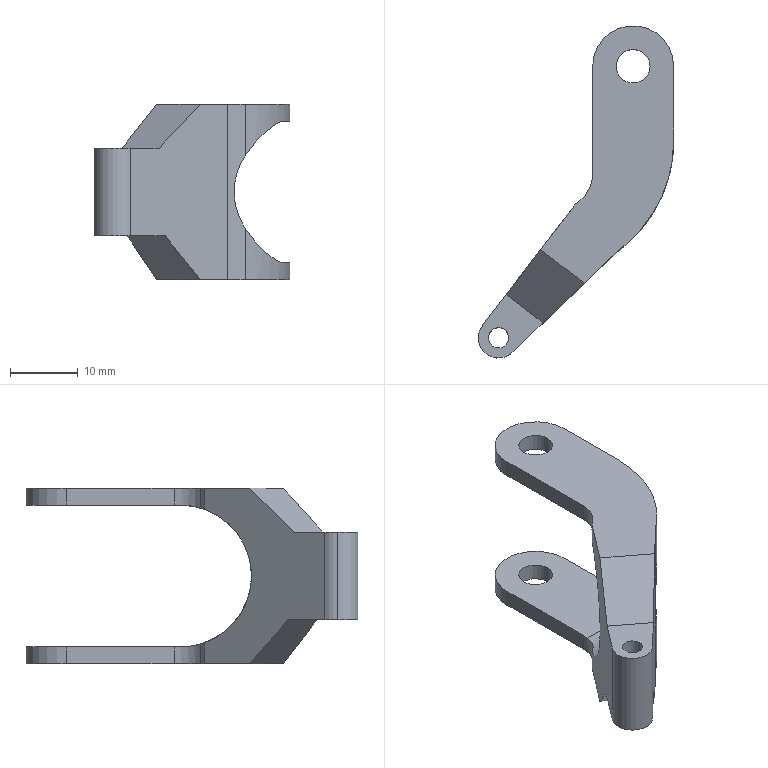Part | SolidWorks | features BaseBody 1 | 1 solid | 32 faces | box 28.933 x 49.206 x 26 mm | volume 4873 mm3 | plane 17 | cylinder 15 | commonest cylinder face diameters 5 x4 3 x2 6 x2 10 x2 12 x2 40 x2
STEP:
#1=CARTESIAN_POINT('',(6.042,20.411,23.5));
#2=VERTEX_POINT('',#1);
#3=CARTESIAN_POINT('',(11.042,20.411,23.5));
#4=VERTEX_POINT('',#3);
#5=CARTESIAN_POINT('',(8.542,20.411,23.5));
#6=DIRECTION('',(0.,0.,1.));
#7=DIRECTION('',(1.,0.,0.));
#8=AXIS2_PLACEMENT_3D('',#5,#6,#7);
#9=CIRCLE('',#8,2.5);
#10=EDGE_CURVE('',#2,#4,#9,.T.);
#11=ORIENTED_EDGE('',*,*,#10,.F.);
#12=CARTESIAN_POINT('',(6.042,20.411,26.));
#13=VERTEX_POINT('',#12);
#14=CARTESIAN_POINT('',(6.042,20.411,-34.));
#15=DIRECTION('',(0.,0.,1.));
#16=VECTOR('',#15,1000.);
#17=LINE('',#14,#16);
#18=EDGE_CURVE('',#2,#13,#17,.T.);
#19=ORIENTED_EDGE('',*,*,#18,.T.);
#20=CARTESIAN_POINT('',(11.042,20.411,26.));
#21=VERTEX_POINT('',#20);
#22=CARTESIAN_POINT('',(8.542,20.411,26.));
#23=DIRECTION('',(0.,0.,1.));
#24=DIRECTION('',(1.,0.,0.));
#25=AXIS2_PLACEMENT_3D('',#22,#23,#24);
#26=CIRCLE('',#25,2.5);
#27=EDGE_CURVE('',#13,#21,#26,.T.);
#28=ORIENTED_EDGE('',*,*,#27,.T.);
#29=CARTESIAN_POINT('',(11.042,20.411,-34.));
#30=DIRECTION('',(0.,0.,1.));
#31=VECTOR('',#30,1000.);
#32=LINE('',#29,#31);
#33=EDGE_CURVE('',#4,#21,#32,.T.);
#34=ORIENTED_EDGE('',*,*,#33,.F.);
#35=EDGE_LOOP('',(#11,#19,#28,#34));
#36=FACE_OUTER_BOUND('',#35,.T.);
#37=CARTESIAN_POINT('',(8.542,20.411,-34.));
#38=DIRECTION('',(0.,0.,1.));
#39=DIRECTION('',(1.,0.,0.));
#40=AXIS2_PLACEMENT_3D('',#37,#38,#39);
#41=CYLINDRICAL_SURFACE('',#40,2.5);
#42=ADVANCED_FACE('',(#36),#41,.F.);
#43=CARTESIAN_POINT('',(11.042,20.411,0.));
#44=VERTEX_POINT('',#43);
#45=CARTESIAN_POINT('',(6.042,20.411,0.));
#46=VERTEX_POINT('',#45);
#47=CARTESIAN_POINT('',(8.542,20.411,0.));
#48=DIRECTION('',(0.,0.,-1.));
#49=DIRECTION('',(-1.,0.,0.));
#50=AXIS2_PLACEMENT_3D('',#47,#48,#49);
#51=CIRCLE('',#50,2.5);
#52=EDGE_CURVE('',#44,#46,#51,.T.);
#53=ORIENTED_EDGE('',*,*,#52,.T.);
#54=CARTESIAN_POINT('',(6.042,20.411,2.5));
#55=VERTEX_POINT('',#54);
#56=CARTESIAN_POINT('',(6.042,20.411,-34.));
#57=DIRECTION('',(0.,0.,1.));
#58=VECTOR('',#57,1000.);
#59=LINE('',#56,#58);
#60=EDGE_CURVE('',#46,#55,#59,.T.);
#61=ORIENTED_EDGE('',*,*,#60,.T.);
#62=CARTESIAN_POINT('',(11.042,20.411,2.5));
#63=VERTEX_POINT('',#62);
#64=CARTESIAN_POINT('',(8.542,20.411,2.5));
#65=DIRECTION('',(0.,0.,-1.));
#66=DIRECTION('',(0.,1.,0.));
#67=AXIS2_PLACEMENT_3D('',#64,#65,#66);
#68=CIRCLE('',#67,2.5);
#69=EDGE_CURVE('',#63,#55,#68,.T.);
#70=ORIENTED_EDGE('',*,*,#69,.F.);
#71=CARTESIAN_POINT('',(11.042,20.411,-34.));
#72=DIRECTION('',(0.,0.,1.));
#73=VECTOR('',#72,1000.);
#74=LINE('',#71,#73);
#75=EDGE_CURVE('',#44,#63,#74,.T.);
#76=ORIENTED_EDGE('',*,*,#75,.F.);
#77=EDGE_LOOP('',(#53,#61,#70,#76));
#78=FACE_OUTER_BOUND('',#77,.T.);
#79=CARTESIAN_POINT('',(8.542,20.411,-34.));
#80=DIRECTION('',(0.,0.,1.));
#81=DIRECTION('',(1.,0.,0.));
#82=AXIS2_PLACEMENT_3D('',#79,#80,#81);
#83=CYLINDRICAL_SURFACE('',#82,2.5);
#84=ADVANCED_FACE('',(#78),#83,.F.);
#85=CARTESIAN_POINT('',(-12.891,-19.795,6.5));
#86=VERTEX_POINT('',#85);
#87=CARTESIAN_POINT('',(-9.891,-19.795,6.5));
#88=VERTEX_POINT('',#87);
#89=CARTESIAN_POINT('',(-11.391,-19.795,6.5));
#90=DIRECTION('',(0.,0.,1.));
#91=DIRECTION('',(1.,0.,0.));
#92=AXIS2_PLACEMENT_3D('',#89,#90,#91);
#93=CIRCLE('',#92,1.5);
#94=EDGE_CURVE('',#86,#88,#93,.T.);
#95=ORIENTED_EDGE('',*,*,#94,.F.);
#96=CARTESIAN_POINT('',(-12.891,-19.795,19.5));
#97=VERTEX_POINT('',#96);
#98=CARTESIAN_POINT('',(-12.891,-19.795,-34.));
#99=DIRECTION('',(0.,0.,1.));
#100=VECTOR('',#99,1000.);
#101=LINE('',#98,#100);
#102=EDGE_CURVE('',#86,#97,#101,.T.);
#103=ORIENTED_EDGE('',*,*,#102,.T.);
#104=CARTESIAN_POINT('',(-9.891,-19.795,19.5));
#105=VERTEX_POINT('',#104);
#106=CARTESIAN_POINT('',(-11.391,-19.795,19.5));
#107=DIRECTION('',(0.,0.,-1.));
#108=DIRECTION('',(-1.,0.,0.));
#109=AXIS2_PLACEMENT_3D('',#106,#107,#108);
#110=CIRCLE('',#109,1.5);
#111=EDGE_CURVE('',#105,#97,#110,.T.);
#112=ORIENTED_EDGE('',*,*,#111,.F.);
#113=CARTESIAN_POINT('',(-9.891,-19.795,-34.));
#114=DIRECTION('',(0.,0.,1.));
#115=VECTOR('',#114,1000.);
#116=LINE('',#113,#115);
#117=EDGE_CURVE('',#88,#105,#116,.T.);
#118=ORIENTED_EDGE('',*,*,#117,.F.);
#119=EDGE_LOOP('',(#95,#103,#112,#118));
#120=FACE_OUTER_BOUND('',#119,.T.);
#121=CARTESIAN_POINT('',(-11.391,-19.795,-34.));
#122=DIRECTION('',(0.,0.,1.));
#123=DIRECTION('',(1.,0.,0.));
#124=AXIS2_PLACEMENT_3D('',#121,#122,#123);
#125=CYLINDRICAL_SURFACE('',#124,1.5);
#126=ADVANCED_FACE('',(#120),#125,.F.);
#127=CARTESIAN_POINT('',(-9.059,-21.682,19.5));
#128=VERTEX_POINT('',#127);
#129=CARTESIAN_POINT('',(-14.391,-19.795,19.5));
#130=VERTEX_POINT('',#129);
#131=CARTESIAN_POINT('',(-11.391,-19.795,19.5));
#132=DIRECTION('',(0.,0.,-1.));
#133=DIRECTION('',(-1.,0.,0.));
#134=AXIS2_PLACEMENT_3D('',#131,#132,#133);
#135=CIRCLE('',#134,3.);
#136=EDGE_CURVE('',#128,#130,#135,.T.);
#137=ORIENTED_EDGE('',*,*,#136,.T.);
#138=CARTESIAN_POINT('',(-14.391,-19.795,6.5));
#139=VERTEX_POINT('',#138);
#140=CARTESIAN_POINT('',(-14.391,-19.795,26.));
#141=DIRECTION('',(0.,0.,-1.));
#142=VECTOR('',#141,1000.);
#143=LINE('',#140,#142);
#144=EDGE_CURVE('',#130,#139,#143,.T.);
#145=ORIENTED_EDGE('',*,*,#144,.T.);
#146=CARTESIAN_POINT('',(-9.059,-21.682,6.5));
#147=VERTEX_POINT('',#146);
#148=CARTESIAN_POINT('',(-11.391,-19.795,6.5));
#149=DIRECTION('',(0.,0.,1.));
#150=DIRECTION('',(1.,0.,0.));
#151=AXIS2_PLACEMENT_3D('',#148,#149,#150);
#152=CIRCLE('',#151,3.);
#153=EDGE_CURVE('',#139,#147,#152,.T.);
#154=ORIENTED_EDGE('',*,*,#153,.T.);
#155=CARTESIAN_POINT('',(-9.059,-21.682,26.));
#156=DIRECTION('',(0.,0.,-1.));
#157=VECTOR('',#156,1000.);
#158=LINE('',#155,#157);
#159=EDGE_CURVE('',#128,#147,#158,.T.);
#160=ORIENTED_EDGE('',*,*,#159,.F.);
#161=EDGE_LOOP('',(#137,#145,#154,#160));
#162=FACE_OUTER_BOUND('',#161,.T.);
#163=CARTESIAN_POINT('',(-11.391,-19.795,26.));
#164=DIRECTION('',(0.,0.,-1.));
#165=DIRECTION('',(-1.,0.,0.));
#166=AXIS2_PLACEMENT_3D('',#163,#164,#165);
#167=CYLINDRICAL_SURFACE('',#166,3.);
#168=ADVANCED_FACE('',(#162),#167,.T.);
#169=CARTESIAN_POINT('',(14.542,9.306,26.));
#170=VERTEX_POINT('',#169);
#171=CARTESIAN_POINT('',(14.542,20.411,26.));
#172=VERTEX_POINT('',#171);
#173=CARTESIAN_POINT('',(14.542,20.411,26.));
#174=DIRECTION('',(0.,1.,0.));
#175=VECTOR('',#174,1000.);
#176=LINE('',#173,#175);
#177=EDGE_CURVE('',#170,#172,#176,.T.);
#178=ORIENTED_EDGE('',*,*,#177,.F.);
#179=CARTESIAN_POINT('',(14.542,9.306,23.5));
#180=VERTEX_POINT('',#179);
#181=CARTESIAN_POINT('',(14.542,9.306,26.));
#182=DIRECTION('',(0.,0.,-1.));
#183=VECTOR('',#182,1000.);
#184=LINE('',#181,#183);
#185=EDGE_CURVE('',#170,#180,#184,.T.);
#186=ORIENTED_EDGE('',*,*,#185,.T.);
#187=CARTESIAN_POINT('',(14.542,20.411,23.5));
#188=VERTEX_POINT('',#187);
#189=CARTESIAN_POINT('',(14.542,20.411,23.5));
#190=DIRECTION('',(0.,1.,0.));
#191=VECTOR('',#190,1000.);
#192=LINE('',#189,#191);
#193=EDGE_CURVE('',#180,#188,#192,.T.);
#194=ORIENTED_EDGE('',*,*,#193,.T.);
#195=CARTESIAN_POINT('',(14.542,20.411,26.));
#196=DIRECTION('',(0.,0.,-1.));
#197=VECTOR('',#196,1000.);
#198=LINE('',#195,#197);
#199=EDGE_CURVE('',#172,#188,#198,.T.);
#200=ORIENTED_EDGE('',*,*,#199,.F.);
#201=EDGE_LOOP('',(#178,#186,#194,#200));
#202=FACE_OUTER_BOUND('',#201,.T.);
#203=CARTESIAN_POINT('',(14.542,20.411,26.));
#204=DIRECTION('',(-1.,0.,0.));
#205=DIRECTION('',(0.,-1.,0.));
#206=AXIS2_PLACEMENT_3D('',#203,#204,#205);
#207=PLANE('',#206);
#208=ADVANCED_FACE('',(#202),#207,.F.);
#209=ORIENTED_EDGE('',*,*,#199,.T.);
#210=CARTESIAN_POINT('',(2.542,20.411,23.5));
#211=VERTEX_POINT('',#210);
#212=CARTESIAN_POINT('',(8.542,20.411,23.5));
#213=DIRECTION('',(0.,0.,1.));
#214=DIRECTION('',(1.,0.,0.));
#215=AXIS2_PLACEMENT_3D('',#212,#213,#214);
#216=CIRCLE('',#215,6.);
#217=EDGE_CURVE('',#188,#211,#216,.T.);
#218=ORIENTED_EDGE('',*,*,#217,.T.);
#219=CARTESIAN_POINT('',(2.542,20.411,26.));
#220=VERTEX_POINT('',#219);
#221=CARTESIAN_POINT('',(2.542,20.411,26.));
#222=DIRECTION('',(0.,0.,-1.));
#223=VECTOR('',#222,1000.);
#224=LINE('',#221,#223);
#225=EDGE_CURVE('',#220,#211,#224,.T.);
#226=ORIENTED_EDGE('',*,*,#225,.F.);
#227=CARTESIAN_POINT('',(8.542,20.411,26.));
#228=DIRECTION('',(0.,0.,1.));
#229=DIRECTION('',(-1.,0.,0.));
#230=AXIS2_PLACEMENT_3D('',#227,#228,#229);
#231=CIRCLE('',#230,6.);
#232=EDGE_CURVE('',#172,#220,#231,.T.);
#233=ORIENTED_EDGE('',*,*,#232,.F.);
#234=EDGE_LOOP('',(#209,#218,#226,#233));
#235=FACE_OUTER_BOUND('',#234,.T.);
#236=CARTESIAN_POINT('',(8.542,20.411,26.));
#237=DIRECTION('',(0.,0.,-1.));
#238=DIRECTION('',(-1.,0.,0.));
#239=AXIS2_PLACEMENT_3D('',#236,#237,#238);
#240=CYLINDRICAL_SURFACE('',#239,6.);
#241=ADVANCED_FACE('',(#235),#240,.T.);
#242=CARTESIAN_POINT('',(2.542,4.432,23.5));
#243=VERTEX_POINT('',#242);
#244=CARTESIAN_POINT('',(2.542,2.016,23.5));
#245=DIRECTION('',(0.,-1.,0.));
#246=VECTOR('',#245,1000.);
#247=LINE('',#244,#246);
#248=EDGE_CURVE('',#211,#243,#247,.T.);
#249=ORIENTED_EDGE('',*,*,#248,.T.);
#250=CARTESIAN_POINT('',(2.542,4.432,26.));
#251=VERTEX_POINT('',#250);
#252=CARTESIAN_POINT('',(2.542,4.432,26.));
#253=DIRECTION('',(0.,0.,1.));
#254=VECTOR('',#253,1000.);
#255=LINE('',#252,#254);
#256=EDGE_CURVE('',#243,#251,#255,.T.);
#257=ORIENTED_EDGE('',*,*,#256,.T.);
#258=CARTESIAN_POINT('',(2.542,2.016,26.));
#259=DIRECTION('',(0.,-1.,0.));
#260=VECTOR('',#259,1000.);
#261=LINE('',#258,#260);
#262=EDGE_CURVE('',#220,#251,#261,.T.);
#263=ORIENTED_EDGE('',*,*,#262,.F.);
#264=ORIENTED_EDGE('',*,*,#225,.T.);
#265=EDGE_LOOP('',(#249,#257,#263,#264));
#266=FACE_OUTER_BOUND('',#265,.T.);
#267=CARTESIAN_POINT('',(2.542,2.016,26.));
#268=DIRECTION('',(1.,0.,0.));
#269=DIRECTION('',(0.,0.,-1.));
#270=AXIS2_PLACEMENT_3D('',#267,#268,#269);
#271=PLANE('',#270);
#272=ADVANCED_FACE('',(#266),#271,.F.);
#273=CARTESIAN_POINT('',(0.,0.,3.098));
#274=VERTEX_POINT('',#273);
#275=CARTESIAN_POINT('',(0.649,0.5148,2.931));
#276=VERTEX_POINT('',#275);
#277=CARTESIAN_POINT('',(0.,0.,3.098));
#278=CARTESIAN_POINT('',(0.2145,0.1702,3.038));
#279=CARTESIAN_POINT('',(0.4309,0.3418,2.982));
#280=CARTESIAN_POINT('',(0.649,0.5148,2.931));
#281=(BOUNDED_CURVE()B_SPLINE_CURVE(3,(#277,#278,#279,#280),.UNSPECIFIED.,.F.,.T.)B_SPLINE_CURVE_WITH_KNOTS((4,4),(1.232,1.283),.UNSPECIFIED.)CURVE()GEOMETRIC_REPRESENTATION_ITEM()RATIONAL_B_SPLINE_CURVE((1.,0.9998,0.9998,1.))REPRESENTATION_ITEM(''));
#282=EDGE_CURVE('',#274,#276,#281,.T.);
#283=ORIENTED_EDGE('',*,*,#282,.T.);
#284=CARTESIAN_POINT('',(0.649,0.5148,0.));
#285=VERTEX_POINT('',#284);
#286=CARTESIAN_POINT('',(0.649,0.5148,0.));
#287=DIRECTION('',(0.,0.,-1.));
#288=VECTOR('',#287,1000.);
#289=LINE('',#286,#288);
#290=EDGE_CURVE('',#276,#285,#289,.T.);
#291=ORIENTED_EDGE('',*,*,#290,.T.);
#292=CARTESIAN_POINT('',(0.,0.,0.));
#293=VERTEX_POINT('',#292);
#294=CARTESIAN_POINT('',(0.,0.,0.));
#295=DIRECTION('',(-0.7835,-0.6214,0.));
#296=VECTOR('',#295,1000.);
#297=LINE('',#294,#296);
#298=EDGE_CURVE('',#285,#293,#297,.T.);
#299=ORIENTED_EDGE('',*,*,#298,.T.);
#300=CARTESIAN_POINT('',(0.,0.,26.));
#301=DIRECTION('',(0.,0.,-1.));
#302=VECTOR('',#301,1000.);
#303=LINE('',#300,#302);
#304=EDGE_CURVE('',#274,#293,#303,.T.);
#305=ORIENTED_EDGE('',*,*,#304,.F.);
#306=EDGE_LOOP('',(#283,#291,#299,#305));
#307=FACE_OUTER_BOUND('',#306,.T.);
#308=CARTESIAN_POINT('',(0.,0.,26.));
#309=DIRECTION('',(0.6214,-0.7835,0.));
#310=DIRECTION('',(0.7835,0.6214,0.));
#311=AXIS2_PLACEMENT_3D('',#308,#309,#310);
#312=PLANE('',#311);
#313=ADVANCED_FACE('',(#307),#312,.F.);
#314=CARTESIAN_POINT('',(-13.723,-17.908,19.5));
#315=VERTEX_POINT('',#314);
#316=CARTESIAN_POINT('',(-10.272,-13.404,19.5));
#317=VERTEX_POINT('',#316);
#318=CARTESIAN_POINT('',(-13.723,-17.908,19.5));
#319=DIRECTION('',(0.6083,0.7937,0.));
#320=VECTOR('',#319,1000.);
#321=LINE('',#318,#320);
#322=EDGE_CURVE('',#315,#317,#321,.T.);
#323=ORIENTED_EDGE('',*,*,#322,.T.);
#324=CARTESIAN_POINT('',(-5.178,-6.757,26.));
#325=VERTEX_POINT('',#324);
#326=CARTESIAN_POINT('',(-10.272,-13.404,19.5));
#327=DIRECTION('',(-0.4805,-0.627,-0.6132));
#328=VECTOR('',#327,1000.);
#329=LINE('',#326,#328);
#330=EDGE_CURVE('',#325,#317,#329,.T.);
#331=ORIENTED_EDGE('',*,*,#330,.F.);
#332=CARTESIAN_POINT('',(0.,0.,26.));
#333=VERTEX_POINT('',#332);
#334=CARTESIAN_POINT('',(-13.723,-17.908,26.));
#335=DIRECTION('',(-0.6083,-0.7937,0.));
#336=VECTOR('',#335,1000.);
#337=LINE('',#334,#336);
#338=EDGE_CURVE('',#333,#325,#337,.T.);
#339=ORIENTED_EDGE('',*,*,#338,.F.);
#340=CARTESIAN_POINT('',(0.,0.,22.902));
#341=VERTEX_POINT('',#340);
#342=CARTESIAN_POINT('',(0.,0.,26.));
#343=DIRECTION('',(0.,0.,-1.));
#344=VECTOR('',#343,1000.);
#345=LINE('',#342,#344);
#346=EDGE_CURVE('',#333,#341,#345,.T.);
#347=ORIENTED_EDGE('',*,*,#346,.T.);
#348=CARTESIAN_POINT('',(0.,0.,22.902));
#349=CARTESIAN_POINT('',(-8.596,-11.217,18.947));
#350=CARTESIAN_POINT('',(-8.596,-11.217,7.053));
#351=CARTESIAN_POINT('',(0.,0.,3.098));
#352=(BOUNDED_CURVE()B_SPLINE_CURVE(3,(#348,#349,#350,#351),.UNSPECIFIED.,.F.,.F.)B_SPLINE_CURVE_WITH_KNOTS((4,4),(5.051,7.515),.UNSPECIFIED.)CURVE()GEOMETRIC_REPRESENTATION_ITEM()RATIONAL_B_SPLINE_CURVE((1.,0.555,0.555,1.))REPRESENTATION_ITEM(''));
#353=EDGE_CURVE('',#341,#274,#352,.T.);
#354=ORIENTED_EDGE('',*,*,#353,.T.);
#355=ORIENTED_EDGE('',*,*,#304,.T.);
#356=CARTESIAN_POINT('',(-5.178,-6.757,0.));
#357=VERTEX_POINT('',#356);
#358=CARTESIAN_POINT('',(-13.723,-17.908,0.));
#359=DIRECTION('',(-0.6083,-0.7937,0.));
#360=VECTOR('',#359,1000.);
#361=LINE('',#358,#360);
#362=EDGE_CURVE('',#293,#357,#361,.T.);
#363=ORIENTED_EDGE('',*,*,#362,.T.);
#364=CARTESIAN_POINT('',(-9.514,-12.415,6.5));
#365=VERTEX_POINT('',#364);
#366=CARTESIAN_POINT('',(-17.717,-23.12,18.8));
#367=DIRECTION('',(-0.4494,-0.5865,0.6738));
#368=VECTOR('',#367,1000.);
#369=LINE('',#366,#368);
#370=EDGE_CURVE('',#357,#365,#369,.T.);
#371=ORIENTED_EDGE('',*,*,#370,.T.);
#372=CARTESIAN_POINT('',(-13.723,-17.908,6.5));
#373=VERTEX_POINT('',#372);
#374=CARTESIAN_POINT('',(-13.723,-17.908,6.5));
#375=DIRECTION('',(-0.6083,-0.7937,0.));
#376=VECTOR('',#375,1000.);
#377=LINE('',#374,#376);
#378=EDGE_CURVE('',#365,#373,#377,.T.);
#379=ORIENTED_EDGE('',*,*,#378,.T.);
#380=CARTESIAN_POINT('',(-13.723,-17.908,26.));
#381=DIRECTION('',(0.,0.,-1.));
#382=VECTOR('',#381,1000.);
#383=LINE('',#380,#382);
#384=EDGE_CURVE('',#315,#373,#383,.T.);
#385=ORIENTED_EDGE('',*,*,#384,.F.);
#386=EDGE_LOOP('',(#323,#331,#339,#347,#354,#355,#363,#371,#379,#385));
#387=FACE_OUTER_BOUND('',#386,.T.);
#388=CARTESIAN_POINT('',(-13.723,-17.908,26.));
#389=DIRECTION('',(0.7937,-0.6083,0.));
#390=DIRECTION('',(0.6083,0.7937,0.));
#391=AXIS2_PLACEMENT_3D('',#388,#389,#390);
#392=PLANE('',#391);
#393=ADVANCED_FACE('',(#387),#392,.F.);
#394=ORIENTED_EDGE('',*,*,#144,.F.);
#395=CARTESIAN_POINT('',(-11.391,-19.795,19.5));
#396=DIRECTION('',(0.,0.,-1.));
#397=DIRECTION('',(-1.,0.,0.));
#398=AXIS2_PLACEMENT_3D('',#395,#396,#397);
#399=CIRCLE('',#398,3.);
#400=EDGE_CURVE('',#130,#315,#399,.T.);
#401=ORIENTED_EDGE('',*,*,#400,.T.);
#402=ORIENTED_EDGE('',*,*,#384,.T.);
#403=CARTESIAN_POINT('',(-11.391,-19.795,6.5));
#404=DIRECTION('',(0.,0.,1.));
#405=DIRECTION('',(1.,0.,0.));
#406=AXIS2_PLACEMENT_3D('',#403,#404,#405);
#407=CIRCLE('',#406,3.);
#408=EDGE_CURVE('',#373,#139,#407,.T.);
#409=ORIENTED_EDGE('',*,*,#408,.T.);
#410=EDGE_LOOP('',(#394,#401,#402,#409));
#411=FACE_OUTER_BOUND('',#410,.T.);
#412=CARTESIAN_POINT('',(-11.391,-19.795,26.));
#413=DIRECTION('',(0.,0.,-1.));
#414=DIRECTION('',(-1.,0.,0.));
#415=AXIS2_PLACEMENT_3D('',#412,#413,#414);
#416=CYLINDRICAL_SURFACE('',#415,3.);
#417=ADVANCED_FACE('',(#411),#416,.T.);
#418=CARTESIAN_POINT('',(1.322,-11.739,26.));
#419=VERTEX_POINT('',#418);
#420=CARTESIAN_POINT('',(-4.797,-17.599,19.5));
#421=VERTEX_POINT('',#420);
#422=CARTESIAN_POINT('',(-5.213,-17.998,19.058));
#423=DIRECTION('',(-0.573,-0.5488,-0.6087));
#424=VECTOR('',#423,1000.);
#425=LINE('',#422,#424);
#426=EDGE_CURVE('',#419,#421,#425,.T.);
#427=ORIENTED_EDGE('',*,*,#426,.T.);
#428=CARTESIAN_POINT('',(-9.059,-21.682,19.5));
#429=DIRECTION('',(-0.7221,-0.6917,0.));
#430=VECTOR('',#429,1000.);
#431=LINE('',#428,#430);
#432=EDGE_CURVE('',#421,#128,#431,.T.);
#433=ORIENTED_EDGE('',*,*,#432,.T.);
#434=ORIENTED_EDGE('',*,*,#159,.T.);
#435=CARTESIAN_POINT('',(-3.886,-16.727,6.5));
#436=VERTEX_POINT('',#435);
#437=CARTESIAN_POINT('',(-9.059,-21.682,6.5));
#438=DIRECTION('',(0.7221,0.6917,0.));
#439=VECTOR('',#438,1000.);
#440=LINE('',#437,#439);
#441=EDGE_CURVE('',#147,#436,#440,.T.);
#442=ORIENTED_EDGE('',*,*,#441,.T.);
#443=CARTESIAN_POINT('',(1.322,-11.739,0.));
#444=VERTEX_POINT('',#443);
#445=CARTESIAN_POINT('',(-13.744,-26.17,18.803));
#446=DIRECTION('',(0.5364,0.5138,-0.6695));
#447=VECTOR('',#446,1000.);
#448=LINE('',#445,#447);
#449=EDGE_CURVE('',#436,#444,#448,.T.);
#450=ORIENTED_EDGE('',*,*,#449,.T.);
#451=CARTESIAN_POINT('',(5.384,-7.848,0.));
#452=VERTEX_POINT('',#451);
#453=CARTESIAN_POINT('',(-9.059,-21.682,0.));
#454=DIRECTION('',(0.7221,0.6917,0.));
#455=VECTOR('',#454,1000.);
#456=LINE('',#453,#455);
#457=EDGE_CURVE('',#444,#452,#456,.T.);
#458=ORIENTED_EDGE('',*,*,#457,.T.);
#459=CARTESIAN_POINT('',(5.384,-7.848,26.));
#460=VERTEX_POINT('',#459);
#461=CARTESIAN_POINT('',(5.384,-7.848,26.));
#462=DIRECTION('',(0.,0.,-1.));
#463=VECTOR('',#462,1000.);
#464=LINE('',#461,#463);
#465=EDGE_CURVE('',#460,#452,#464,.T.);
#466=ORIENTED_EDGE('',*,*,#465,.F.);
#467=CARTESIAN_POINT('',(-9.059,-21.682,26.));
#468=DIRECTION('',(0.7221,0.6917,0.));
#469=VECTOR('',#468,1000.);
#470=LINE('',#467,#469);
#471=EDGE_CURVE('',#419,#460,#470,.T.);
#472=ORIENTED_EDGE('',*,*,#471,.F.);
#473=EDGE_LOOP('',(#427,#433,#434,#442,#450,#458,#466,#472));
#474=FACE_OUTER_BOUND('',#473,.T.);
#475=CARTESIAN_POINT('',(-9.059,-21.682,26.));
#476=DIRECTION('',(-0.6917,0.7221,0.));
#477=DIRECTION('',(-0.7221,-0.6917,0.));
#478=AXIS2_PLACEMENT_3D('',#475,#476,#477);
#479=PLANE('',#478);
#480=ADVANCED_FACE('',(#474),#479,.F.);
#481=CARTESIAN_POINT('',(7.936,-5.546,0.));
#482=VERTEX_POINT('',#481);
#483=CARTESIAN_POINT('',(5.384,-7.848,0.));
#484=DIRECTION('',(0.7426,0.6697,0.));
#485=VECTOR('',#484,1000.);
#486=LINE('',#483,#485);
#487=EDGE_CURVE('',#452,#482,#486,.T.);
#488=ORIENTED_EDGE('',*,*,#487,.T.);
#489=CARTESIAN_POINT('',(7.936,-5.546,7.656));
#490=VERTEX_POINT('',#489);
#491=CARTESIAN_POINT('',(7.936,-5.546,26.));
#492=DIRECTION('',(0.,0.,1.));
#493=VECTOR('',#492,1000.);
#494=LINE('',#491,#493);
#495=EDGE_CURVE('',#482,#490,#494,.T.);
#496=ORIENTED_EDGE('',*,*,#495,.T.);
#497=CARTESIAN_POINT('',(7.936,-5.546,18.344));
#498=VERTEX_POINT('',#497);
#499=CARTESIAN_POINT('',(7.936,-5.546,7.656));
#500=CARTESIAN_POINT('',(5.719,-7.546,11.036));
#501=CARTESIAN_POINT('',(5.719,-7.546,14.964));
#502=CARTESIAN_POINT('',(7.936,-5.546,18.344));
#503=(BOUNDED_CURVE()B_SPLINE_CURVE(3,(#499,#500,#501,#502),.UNSPECIFIED.,.F.,.F.)B_SPLINE_CURVE_WITH_KNOTS((4,4),(5.749,6.817),.UNSPECIFIED.)CURVE()GEOMETRIC_REPRESENTATION_ITEM()RATIONAL_B_SPLINE_CURVE((1.,0.9072,0.9072,1.))REPRESENTATION_ITEM(''));
#504=EDGE_CURVE('',#490,#498,#503,.T.);
#505=ORIENTED_EDGE('',*,*,#504,.T.);
#506=CARTESIAN_POINT('',(7.936,-5.546,26.));
#507=VERTEX_POINT('',#506);
#508=CARTESIAN_POINT('',(7.936,-5.546,26.));
#509=DIRECTION('',(0.,0.,1.));
#510=VECTOR('',#509,1000.);
#511=LINE('',#508,#510);
#512=EDGE_CURVE('',#498,#507,#511,.T.);
#513=ORIENTED_EDGE('',*,*,#512,.T.);
#514=CARTESIAN_POINT('',(5.384,-7.848,26.));
#515=DIRECTION('',(0.7426,0.6697,0.));
#516=VECTOR('',#515,1000.);
#517=LINE('',#514,#516);
#518=EDGE_CURVE('',#460,#507,#517,.T.);
#519=ORIENTED_EDGE('',*,*,#518,.F.);
#520=ORIENTED_EDGE('',*,*,#465,.T.);
#521=EDGE_LOOP('',(#488,#496,#505,#513,#519,#520));
#522=FACE_OUTER_BOUND('',#521,.T.);
#523=CARTESIAN_POINT('',(5.384,-7.848,26.));
#524=DIRECTION('',(-0.6697,0.7426,0.));
#525=DIRECTION('',(-0.7426,-0.6697,0.));
#526=AXIS2_PLACEMENT_3D('',#523,#524,#525);
#527=PLANE('',#526);
#528=ADVANCED_FACE('',(#522),#527,.F.);
#529=CARTESIAN_POINT('',(14.542,20.411,2.5));
#530=VERTEX_POINT('',#529);
#531=CARTESIAN_POINT('',(14.542,9.306,2.5));
#532=VERTEX_POINT('',#531);
#533=CARTESIAN_POINT('',(14.542,20.411,2.5));
#534=DIRECTION('',(0.,-1.,0.));
#535=VECTOR('',#534,1000.);
#536=LINE('',#533,#535);
#537=EDGE_CURVE('',#530,#532,#536,.T.);
#538=ORIENTED_EDGE('',*,*,#537,.T.);
#539=CARTESIAN_POINT('',(14.542,9.306,0.));
#540=VERTEX_POINT('',#539);
#541=CARTESIAN_POINT('',(14.542,9.306,26.));
#542=DIRECTION('',(0.,0.,-1.));
#543=VECTOR('',#542,1000.);
#544=LINE('',#541,#543);
#545=EDGE_CURVE('',#532,#540,#544,.T.);
#546=ORIENTED_EDGE('',*,*,#545,.T.);
#547=CARTESIAN_POINT('',(14.542,20.411,0.));
#548=VERTEX_POINT('',#547);
#549=CARTESIAN_POINT('',(14.542,20.411,0.));
#550=DIRECTION('',(0.,1.,0.));
#551=VECTOR('',#550,1000.);
#552=LINE('',#549,#551);
#553=EDGE_CURVE('',#540,#548,#552,.T.);
#554=ORIENTED_EDGE('',*,*,#553,.T.);
#555=CARTESIAN_POINT('',(14.542,20.411,26.));
#556=DIRECTION('',(0.,0.,-1.));
#557=VECTOR('',#556,1000.);
#558=LINE('',#555,#557);
#559=EDGE_CURVE('',#530,#548,#558,.T.);
#560=ORIENTED_EDGE('',*,*,#559,.F.);
#561=EDGE_LOOP('',(#538,#546,#554,#560));
#562=FACE_OUTER_BOUND('',#561,.T.);
#563=CARTESIAN_POINT('',(14.542,20.411,26.));
#564=DIRECTION('',(-1.,0.,0.));
#565=DIRECTION('',(0.,-1.,0.));
#566=AXIS2_PLACEMENT_3D('',#563,#564,#565);
#567=PLANE('',#566);
#568=ADVANCED_FACE('',(#562),#567,.F.);
#569=CARTESIAN_POINT('',(2.542,20.411,2.5));
#570=VERTEX_POINT('',#569);
#571=CARTESIAN_POINT('',(2.542,20.411,0.));
#572=VERTEX_POINT('',#571);
#573=CARTESIAN_POINT('',(2.542,20.411,26.));
#574=DIRECTION('',(0.,0.,-1.));
#575=VECTOR('',#574,1000.);
#576=LINE('',#573,#575);
#577=EDGE_CURVE('',#570,#572,#576,.T.);
#578=ORIENTED_EDGE('',*,*,#577,.F.);
#579=CARTESIAN_POINT('',(8.542,20.411,2.5));
#580=DIRECTION('',(0.,0.,-1.));
#581=DIRECTION('',(0.,1.,0.));
#582=AXIS2_PLACEMENT_3D('',#579,#580,#581);
#583=CIRCLE('',#582,6.);
#584=EDGE_CURVE('',#570,#530,#583,.T.);
#585=ORIENTED_EDGE('',*,*,#584,.T.);
#586=ORIENTED_EDGE('',*,*,#559,.T.);
#587=CARTESIAN_POINT('',(8.542,20.411,0.));
#588=DIRECTION('',(0.,0.,1.));
#589=DIRECTION('',(-1.,0.,0.));
#590=AXIS2_PLACEMENT_3D('',#587,#588,#589);
#591=CIRCLE('',#590,6.);
#592=EDGE_CURVE('',#548,#572,#591,.T.);
#593=ORIENTED_EDGE('',*,*,#592,.T.);
#594=EDGE_LOOP('',(#578,#585,#586,#593));
#595=FACE_OUTER_BOUND('',#594,.T.);
#596=CARTESIAN_POINT('',(8.542,20.411,26.));
#597=DIRECTION('',(0.,0.,-1.));
#598=DIRECTION('',(-1.,0.,0.));
#599=AXIS2_PLACEMENT_3D('',#596,#597,#598);
#600=CYLINDRICAL_SURFACE('',#599,6.);
#601=ADVANCED_FACE('',(#595),#600,.T.);
#602=CARTESIAN_POINT('',(2.542,4.432,0.));
#603=VERTEX_POINT('',#602);
#604=CARTESIAN_POINT('',(2.542,2.016,0.));
#605=DIRECTION('',(0.,-1.,0.));
#606=VECTOR('',#605,1000.);
#607=LINE('',#604,#606);
#608=EDGE_CURVE('',#572,#603,#607,.T.);
#609=ORIENTED_EDGE('',*,*,#608,.T.);
#610=CARTESIAN_POINT('',(2.542,4.432,2.5));
#611=VERTEX_POINT('',#610);
#612=CARTESIAN_POINT('',(2.542,4.432,2.604));
#613=DIRECTION('',(0.,0.,1.));
#614=VECTOR('',#613,1000.);
#615=LINE('',#612,#614);
#616=EDGE_CURVE('',#603,#611,#615,.T.);
#617=ORIENTED_EDGE('',*,*,#616,.T.);
#618=CARTESIAN_POINT('',(2.542,2.016,2.5));
#619=DIRECTION('',(0.,1.,0.));
#620=VECTOR('',#619,1000.);
#621=LINE('',#618,#620);
#622=EDGE_CURVE('',#611,#570,#621,.T.);
#623=ORIENTED_EDGE('',*,*,#622,.T.);
#624=ORIENTED_EDGE('',*,*,#577,.T.);
#625=EDGE_LOOP('',(#609,#617,#623,#624));
#626=FACE_OUTER_BOUND('',#625,.T.);
#627=CARTESIAN_POINT('',(2.542,2.016,26.));
#628=DIRECTION('',(1.,0.,0.));
#629=DIRECTION('',(0.,0.,-1.));
#630=AXIS2_PLACEMENT_3D('',#627,#628,#629);
#631=PLANE('',#630);
#632=ADVANCED_FACE('',(#626),#631,.F.);
#633=CARTESIAN_POINT('',(0.649,0.5148,26.));
#634=VERTEX_POINT('',#633);
#635=CARTESIAN_POINT('',(0.,0.,26.));
#636=DIRECTION('',(-0.7835,-0.6214,0.));
#637=VECTOR('',#636,1000.);
#638=LINE('',#635,#637);
#639=EDGE_CURVE('',#634,#333,#638,.T.);
#640=ORIENTED_EDGE('',*,*,#639,.F.);
#641=CARTESIAN_POINT('',(0.649,0.5148,23.069));
#642=VERTEX_POINT('',#641);
#643=CARTESIAN_POINT('',(0.649,0.5148,23.396));
#644=DIRECTION('',(0.,0.,-1.));
#645=VECTOR('',#644,1000.);
#646=LINE('',#643,#645);
#647=EDGE_CURVE('',#634,#642,#646,.T.);
#648=ORIENTED_EDGE('',*,*,#647,.T.);
#649=CARTESIAN_POINT('',(0.649,0.5148,23.069));
#650=CARTESIAN_POINT('',(0.4309,0.3418,23.018));
#651=CARTESIAN_POINT('',(0.2145,0.1702,22.962));
#652=CARTESIAN_POINT('',(0.,0.,22.902));
#653=(BOUNDED_CURVE()B_SPLINE_CURVE(3,(#649,#650,#651,#652),.UNSPECIFIED.,.F.,.F.)B_SPLINE_CURVE_WITH_KNOTS((4,4),(5.,5.051),.UNSPECIFIED.)CURVE()GEOMETRIC_REPRESENTATION_ITEM()RATIONAL_B_SPLINE_CURVE((1.,0.9998,0.9998,1.))REPRESENTATION_ITEM(''));
#654=EDGE_CURVE('',#642,#341,#653,.T.);
#655=ORIENTED_EDGE('',*,*,#654,.T.);
#656=ORIENTED_EDGE('',*,*,#346,.F.);
#657=EDGE_LOOP('',(#640,#648,#655,#656));
#658=FACE_OUTER_BOUND('',#657,.T.);
#659=CARTESIAN_POINT('',(0.,0.,26.));
#660=DIRECTION('',(0.6214,-0.7835,0.));
#661=DIRECTION('',(0.7835,0.6214,0.));
#662=AXIS2_PLACEMENT_3D('',#659,#660,#661);
#663=PLANE('',#662);
#664=ADVANCED_FACE('',(#658),#663,.F.);
#665=CARTESIAN_POINT('',(8.542,20.411,26.));
#666=DIRECTION('',(0.,0.,1.));
#667=DIRECTION('',(1.,0.,0.));
#668=AXIS2_PLACEMENT_3D('',#665,#666,#667);
#669=CIRCLE('',#668,2.5);
#670=EDGE_CURVE('',#21,#13,#669,.T.);
#671=ORIENTED_EDGE('',*,*,#670,.F.);
#672=ORIENTED_EDGE('',*,*,#27,.F.);
#673=EDGE_LOOP('',(#671,#672));
#674=FACE_BOUND('',#673,.T.);
#675=ORIENTED_EDGE('',*,*,#338,.T.);
#676=CARTESIAN_POINT('',(-9.651,-3.33,26.));
#677=DIRECTION('',(0.7937,-0.6083,0.));
#678=VECTOR('',#677,1000.);
#679=LINE('',#676,#678);
#680=EDGE_CURVE('',#325,#419,#679,.T.);
#681=ORIENTED_EDGE('',*,*,#680,.T.);
#682=ORIENTED_EDGE('',*,*,#471,.T.);
#683=ORIENTED_EDGE('',*,*,#518,.T.);
#684=CARTESIAN_POINT('',(-5.458,9.306,26.));
#685=DIRECTION('',(0.,0.,1.));
#686=DIRECTION('',(-1.,0.,0.));
#687=AXIS2_PLACEMENT_3D('',#684,#685,#686);
#688=CIRCLE('',#687,20.);
#689=EDGE_CURVE('',#507,#170,#688,.T.);
#690=ORIENTED_EDGE('',*,*,#689,.T.);
#691=ORIENTED_EDGE('',*,*,#177,.T.);
#692=ORIENTED_EDGE('',*,*,#232,.T.);
#693=ORIENTED_EDGE('',*,*,#262,.T.);
#694=CARTESIAN_POINT('',(-2.458,4.432,26.));
#695=DIRECTION('',(0.,0.,-1.));
#696=DIRECTION('',(-1.,0.,0.));
#697=AXIS2_PLACEMENT_3D('',#694,#695,#696);
#698=CIRCLE('',#697,5.);
#699=EDGE_CURVE('',#251,#634,#698,.T.);
#700=ORIENTED_EDGE('',*,*,#699,.T.);
#701=ORIENTED_EDGE('',*,*,#639,.T.);
#702=EDGE_LOOP('',(#675,#681,#682,#683,#690,#691,#692,#693,#700,#701));
#703=FACE_OUTER_BOUND('',#702,.T.);
#704=CARTESIAN_POINT('',(8.542,20.411,26.));
#705=DIRECTION('',(0.,0.,-1.));
#706=DIRECTION('',(-1.,0.,0.));
#707=AXIS2_PLACEMENT_3D('',#704,#705,#706);
#708=PLANE('',#707);
#709=ADVANCED_FACE('',(#674,#703),#708,.F.);
#710=ORIENTED_EDGE('',*,*,#52,.F.);
#711=CARTESIAN_POINT('',(8.542,20.411,0.));
#712=DIRECTION('',(0.,0.,-1.));
#713=DIRECTION('',(-1.,0.,0.));
#714=AXIS2_PLACEMENT_3D('',#711,#712,#713);
#715=CIRCLE('',#714,2.5);
#716=EDGE_CURVE('',#46,#44,#715,.T.);
#717=ORIENTED_EDGE('',*,*,#716,.F.);
#718=EDGE_LOOP('',(#710,#717));
#719=FACE_BOUND('',#718,.T.);
#720=CARTESIAN_POINT('',(-9.651,-3.33,0.));
#721=DIRECTION('',(0.7937,-0.6083,0.));
#722=VECTOR('',#721,1000.);
#723=LINE('',#720,#722);
#724=EDGE_CURVE('',#357,#444,#723,.T.);
#725=ORIENTED_EDGE('',*,*,#724,.F.);
#726=ORIENTED_EDGE('',*,*,#362,.F.);
#727=ORIENTED_EDGE('',*,*,#298,.F.);
#728=CARTESIAN_POINT('',(-2.458,4.432,0.));
#729=DIRECTION('',(0.,0.,1.));
#730=DIRECTION('',(-1.,0.,0.));
#731=AXIS2_PLACEMENT_3D('',#728,#729,#730);
#732=CIRCLE('',#731,5.);
#733=EDGE_CURVE('',#285,#603,#732,.T.);
#734=ORIENTED_EDGE('',*,*,#733,.T.);
#735=ORIENTED_EDGE('',*,*,#608,.F.);
#736=ORIENTED_EDGE('',*,*,#592,.F.);
#737=ORIENTED_EDGE('',*,*,#553,.F.);
#738=CARTESIAN_POINT('',(-5.458,9.306,0.));
#739=DIRECTION('',(0.,0.,-1.));
#740=DIRECTION('',(-1.,0.,0.));
#741=AXIS2_PLACEMENT_3D('',#738,#739,#740);
#742=CIRCLE('',#741,20.);
#743=EDGE_CURVE('',#540,#482,#742,.T.);
#744=ORIENTED_EDGE('',*,*,#743,.T.);
#745=ORIENTED_EDGE('',*,*,#487,.F.);
#746=ORIENTED_EDGE('',*,*,#457,.F.);
#747=EDGE_LOOP('',(#725,#726,#727,#734,#735,#736,#737,#744,#745,#746));
#748=FACE_OUTER_BOUND('',#747,.T.);
#749=CARTESIAN_POINT('',(8.542,20.411,0.));
#750=DIRECTION('',(0.,0.,-1.));
#751=DIRECTION('',(-1.,0.,0.));
#752=AXIS2_PLACEMENT_3D('',#749,#750,#751);
#753=PLANE('',#752);
#754=ADVANCED_FACE('',(#719,#748),#753,.T.);
#755=CARTESIAN_POINT('',(8.542,20.411,23.5));
#756=DIRECTION('',(0.,0.,1.));
#757=DIRECTION('',(1.,0.,0.));
#758=AXIS2_PLACEMENT_3D('',#755,#756,#757);
#759=CIRCLE('',#758,2.5);
#760=EDGE_CURVE('',#4,#2,#759,.T.);
#761=ORIENTED_EDGE('',*,*,#760,.T.);
#762=ORIENTED_EDGE('',*,*,#10,.T.);
#763=EDGE_LOOP('',(#761,#762));
#764=FACE_BOUND('',#763,.T.);
#765=ORIENTED_EDGE('',*,*,#193,.F.);
#766=CARTESIAN_POINT('',(13.678,3.492,23.5));
#767=VERTEX_POINT('',#766);
#768=CARTESIAN_POINT('',(-5.458,9.306,23.5));
#769=DIRECTION('',(0.,0.,-1.));
#770=DIRECTION('',(1.,0.,0.));
#771=AXIS2_PLACEMENT_3D('',#768,#769,#770);
#772=CIRCLE('',#771,20.);
#773=EDGE_CURVE('',#180,#767,#772,.T.);
#774=ORIENTED_EDGE('',*,*,#773,.T.);
#775=CARTESIAN_POINT('',(2.453,3.492,23.5));
#776=VERTEX_POINT('',#775);
#777=CARTESIAN_POINT('',(32.542,3.492,23.5));
#778=DIRECTION('',(-1.,0.,0.));
#779=VECTOR('',#778,1000.);
#780=LINE('',#777,#779);
#781=EDGE_CURVE('',#767,#776,#780,.T.);
#782=ORIENTED_EDGE('',*,*,#781,.T.);
#783=CARTESIAN_POINT('',(-2.458,4.432,23.5));
#784=DIRECTION('',(0.,0.,1.));
#785=DIRECTION('',(1.,0.,0.));
#786=AXIS2_PLACEMENT_3D('',#783,#784,#785);
#787=CIRCLE('',#786,5.);
#788=EDGE_CURVE('',#776,#243,#787,.T.);
#789=ORIENTED_EDGE('',*,*,#788,.T.);
#790=ORIENTED_EDGE('',*,*,#248,.F.);
#791=ORIENTED_EDGE('',*,*,#217,.F.);
#792=EDGE_LOOP('',(#765,#774,#782,#789,#790,#791));
#793=FACE_OUTER_BOUND('',#792,.T.);
#794=CARTESIAN_POINT('',(32.542,3.492,23.5));
#795=DIRECTION('',(0.,0.,1.));
#796=DIRECTION('',(1.,0.,0.));
#797=AXIS2_PLACEMENT_3D('',#794,#795,#796);
#798=PLANE('',#797);
#799=ADVANCED_FACE('',(#764,#793),#798,.F.);
#800=ORIENTED_EDGE('',*,*,#69,.T.);
#801=CARTESIAN_POINT('',(8.542,20.411,2.5));
#802=DIRECTION('',(0.,0.,-1.));
#803=DIRECTION('',(0.,1.,0.));
#804=AXIS2_PLACEMENT_3D('',#801,#802,#803);
#805=CIRCLE('',#804,2.5);
#806=EDGE_CURVE('',#55,#63,#805,.T.);
#807=ORIENTED_EDGE('',*,*,#806,.T.);
#808=EDGE_LOOP('',(#800,#807));
#809=FACE_BOUND('',#808,.T.);
#810=CARTESIAN_POINT('',(13.678,3.492,2.5));
#811=VERTEX_POINT('',#810);
#812=CARTESIAN_POINT('',(2.453,3.492,2.5));
#813=VERTEX_POINT('',#812);
#814=CARTESIAN_POINT('',(32.542,3.492,2.5));
#815=DIRECTION('',(-1.,0.,0.));
#816=VECTOR('',#815,1000.);
#817=LINE('',#814,#816);
#818=EDGE_CURVE('',#811,#813,#817,.T.);
#819=ORIENTED_EDGE('',*,*,#818,.F.);
#820=CARTESIAN_POINT('',(-5.458,9.306,2.5));
#821=DIRECTION('',(0.,0.,1.));
#822=DIRECTION('',(0.,1.,0.));
#823=AXIS2_PLACEMENT_3D('',#820,#821,#822);
#824=CIRCLE('',#823,20.);
#825=EDGE_CURVE('',#811,#532,#824,.T.);
#826=ORIENTED_EDGE('',*,*,#825,.T.);
#827=ORIENTED_EDGE('',*,*,#537,.F.);
#828=ORIENTED_EDGE('',*,*,#584,.F.);
#829=ORIENTED_EDGE('',*,*,#622,.F.);
#830=CARTESIAN_POINT('',(-2.458,4.432,2.5));
#831=DIRECTION('',(0.,0.,-1.));
#832=DIRECTION('',(0.,1.,0.));
#833=AXIS2_PLACEMENT_3D('',#830,#831,#832);
#834=CIRCLE('',#833,5.);
#835=EDGE_CURVE('',#611,#813,#834,.T.);
#836=ORIENTED_EDGE('',*,*,#835,.T.);
#837=EDGE_LOOP('',(#819,#826,#827,#828,#829,#836));
#838=FACE_OUTER_BOUND('',#837,.T.);
#839=CARTESIAN_POINT('',(32.542,28.318,2.5));
#840=DIRECTION('',(0.,0.,-1.));
#841=DIRECTION('',(0.,1.,0.));
#842=AXIS2_PLACEMENT_3D('',#839,#840,#841);
#843=PLANE('',#842);
#844=ADVANCED_FACE('',(#809,#838),#843,.F.);
#845=ORIENTED_EDGE('',*,*,#504,.F.);
#846=CARTESIAN_POINT('',(7.936,-5.546,7.656));
#847=CARTESIAN_POINT('',(8.447,-5.086,6.876));
#848=CARTESIAN_POINT('',(8.987,-4.55,6.193));
#849=CARTESIAN_POINT('',(9.799,-3.632,5.274));
#850=CARTESIAN_POINT('',(10.069,-3.307,4.986));
#851=CARTESIAN_POINT('',(10.607,-2.614,4.446));
#852=CARTESIAN_POINT('',(10.876,-2.245,4.194));
#853=CARTESIAN_POINT('',(11.649,-1.095,3.513));
#854=CARTESIAN_POINT('',(12.129,-0.2694,3.152));
#855=CARTESIAN_POINT('',(12.777,1.076,2.771));
#856=CARTESIAN_POINT('',(12.982,1.546,2.67));
#857=CARTESIAN_POINT('',(13.357,2.504,2.535));
#858=CARTESIAN_POINT('',(13.526,2.993,2.5));
#859=CARTESIAN_POINT('',(13.678,3.492,2.5));
#860=B_SPLINE_CURVE_WITH_KNOTS('',3,(#846,#847,#848,#849,#850,#851,#852,#853,#854,#855,#856,#857,#858,#859),.UNSPECIFIED.,.F.,.F.,(4,2,2,2,2,2,4),(0.,0.003061,0.004592,0.006122,0.009184,0.01071,0.01224),.UNSPECIFIED.);
#861=EDGE_CURVE('',#490,#811,#860,.T.);
#862=ORIENTED_EDGE('',*,*,#861,.T.);
#863=ORIENTED_EDGE('',*,*,#818,.T.);
#864=CARTESIAN_POINT('',(2.453,3.492,2.5));
#865=CARTESIAN_POINT('',(2.396,3.195,2.5));
#866=CARTESIAN_POINT('',(2.314,2.909,2.512));
#867=CARTESIAN_POINT('',(2.1,2.357,2.558));
#868=CARTESIAN_POINT('',(1.968,2.088,2.591));
#869=CARTESIAN_POINT('',(1.659,1.58,2.672));
#870=CARTESIAN_POINT('',(1.485,1.344,2.72));
#871=CARTESIAN_POINT('',(1.096,0.9035,2.821));
#872=CARTESIAN_POINT('',(0.8812,0.6989,2.876));
#873=CARTESIAN_POINT('',(0.649,0.5148,2.931));
#874=B_SPLINE_CURVE_WITH_KNOTS('',3,(#864,#865,#866,#867,#868,#869,#870,#871,#872,#873),.UNSPECIFIED.,.F.,.F.,(4,2,2,2,4),(0.,0.000891,0.001782,0.002673,0.003564),.UNSPECIFIED.);
#875=EDGE_CURVE('',#813,#276,#874,.T.);
#876=ORIENTED_EDGE('',*,*,#875,.T.);
#877=ORIENTED_EDGE('',*,*,#282,.F.);
#878=ORIENTED_EDGE('',*,*,#353,.F.);
#879=ORIENTED_EDGE('',*,*,#654,.F.);
#880=CARTESIAN_POINT('',(0.649,0.5148,23.069));
#881=CARTESIAN_POINT('',(0.8814,0.6991,23.124));
#882=CARTESIAN_POINT('',(1.094,0.9012,23.178));
#883=CARTESIAN_POINT('',(1.482,1.34,23.28));
#884=CARTESIAN_POINT('',(1.659,1.579,23.328));
#885=CARTESIAN_POINT('',(1.968,2.088,23.409));
#886=CARTESIAN_POINT('',(2.099,2.353,23.442));
#887=CARTESIAN_POINT('',(2.312,2.906,23.487));
#888=CARTESIAN_POINT('',(2.396,3.195,23.5));
#889=CARTESIAN_POINT('',(2.453,3.492,23.5));
#890=B_SPLINE_CURVE_WITH_KNOTS('',3,(#880,#881,#882,#883,#884,#885,#886,#887,#888,#889),.UNSPECIFIED.,.F.,.F.,(4,2,2,2,4),(0.,0.0008924,0.001785,0.002677,0.00357),.UNSPECIFIED.);
#891=EDGE_CURVE('',#642,#776,#890,.T.);
#892=ORIENTED_EDGE('',*,*,#891,.T.);
#893=ORIENTED_EDGE('',*,*,#781,.F.);
#894=CARTESIAN_POINT('',(13.678,3.492,23.5));
#895=CARTESIAN_POINT('',(13.375,2.496,23.5));
#896=CARTESIAN_POINT('',(13.005,1.552,23.362));
#897=CARTESIAN_POINT('',(12.357,0.203,22.983));
#898=CARTESIAN_POINT('',(12.125,-0.2372,22.826));
#899=CARTESIAN_POINT('',(11.644,-1.074,22.466));
#900=CARTESIAN_POINT('',(11.394,-1.474,22.262));
#901=CARTESIAN_POINT('',(10.879,-2.239,21.809));
#902=CARTESIAN_POINT('',(10.613,-2.606,21.56));
#903=CARTESIAN_POINT('',(10.073,-3.303,21.018));
#904=CARTESIAN_POINT('',(9.801,-3.629,20.729));
#905=CARTESIAN_POINT('',(8.987,-4.55,19.807));
#906=CARTESIAN_POINT('',(8.446,-5.086,19.122));
#907=CARTESIAN_POINT('',(7.936,-5.546,18.344));
#908=B_SPLINE_CURVE_WITH_KNOTS('',3,(#894,#895,#896,#897,#898,#899,#900,#901,#902,#903,#904,#905,#906,#907),.UNSPECIFIED.,.F.,.F.,(4,2,2,2,2,2,4),(0.,0.00307,0.004604,0.006139,0.007674,0.009209,0.01228),.UNSPECIFIED.);
#909=EDGE_CURVE('',#767,#498,#908,.T.);
#910=ORIENTED_EDGE('',*,*,#909,.T.);
#911=EDGE_LOOP('',(#845,#862,#863,#876,#877,#878,#879,#892,#893,#910));
#912=FACE_OUTER_BOUND('',#911,.T.);
#913=CARTESIAN_POINT('',(32.542,3.492,13.));
#914=DIRECTION('',(-1.,0.,0.));
#915=DIRECTION('',(0.,0.,1.));
#916=AXIS2_PLACEMENT_3D('',#913,#914,#915);
#917=CYLINDRICAL_SURFACE('',#916,10.5);
#918=ADVANCED_FACE('',(#912),#917,.F.);
#919=ORIENTED_EDGE('',*,*,#861,.F.);
#920=ORIENTED_EDGE('',*,*,#495,.F.);
#921=ORIENTED_EDGE('',*,*,#743,.F.);
#922=ORIENTED_EDGE('',*,*,#545,.F.);
#923=ORIENTED_EDGE('',*,*,#825,.F.);
#924=EDGE_LOOP('',(#919,#920,#921,#922,#923));
#925=FACE_OUTER_BOUND('',#924,.T.);
#926=CARTESIAN_POINT('',(-5.458,9.306,26.));
#927=DIRECTION('',(0.,0.,-1.));
#928=DIRECTION('',(-1.,0.,0.));
#929=AXIS2_PLACEMENT_3D('',#926,#927,#928);
#930=CYLINDRICAL_SURFACE('',#929,20.);
#931=ADVANCED_FACE('',(#925),#930,.T.);
#932=ORIENTED_EDGE('',*,*,#689,.F.);
#933=ORIENTED_EDGE('',*,*,#512,.F.);
#934=ORIENTED_EDGE('',*,*,#909,.F.);
#935=ORIENTED_EDGE('',*,*,#773,.F.);
#936=ORIENTED_EDGE('',*,*,#185,.F.);
#937=EDGE_LOOP('',(#932,#933,#934,#935,#936));
#938=FACE_OUTER_BOUND('',#937,.T.);
#939=CARTESIAN_POINT('',(-5.458,9.306,26.));
#940=DIRECTION('',(0.,0.,-1.));
#941=DIRECTION('',(-1.,0.,0.));
#942=AXIS2_PLACEMENT_3D('',#939,#940,#941);
#943=CYLINDRICAL_SURFACE('',#942,20.);
#944=ADVANCED_FACE('',(#938),#943,.T.);
#945=ORIENTED_EDGE('',*,*,#699,.F.);
#946=ORIENTED_EDGE('',*,*,#256,.F.);
#947=ORIENTED_EDGE('',*,*,#788,.F.);
#948=ORIENTED_EDGE('',*,*,#891,.F.);
#949=ORIENTED_EDGE('',*,*,#647,.F.);
#950=EDGE_LOOP('',(#945,#946,#947,#948,#949));
#951=FACE_OUTER_BOUND('',#950,.T.);
#952=CARTESIAN_POINT('',(-2.458,4.432,26.));
#953=DIRECTION('',(0.,0.,1.));
#954=DIRECTION('',(1.,0.,0.));
#955=AXIS2_PLACEMENT_3D('',#952,#953,#954);
#956=CYLINDRICAL_SURFACE('',#955,5.);
#957=ADVANCED_FACE('',(#951),#956,.F.);
#958=ORIENTED_EDGE('',*,*,#835,.F.);
#959=ORIENTED_EDGE('',*,*,#616,.F.);
#960=ORIENTED_EDGE('',*,*,#733,.F.);
#961=ORIENTED_EDGE('',*,*,#290,.F.);
#962=ORIENTED_EDGE('',*,*,#875,.F.);
#963=EDGE_LOOP('',(#958,#959,#960,#961,#962));
#964=FACE_OUTER_BOUND('',#963,.T.);
#965=CARTESIAN_POINT('',(-2.458,4.432,26.));
#966=DIRECTION('',(0.,0.,1.));
#967=DIRECTION('',(1.,0.,0.));
#968=AXIS2_PLACEMENT_3D('',#965,#966,#967);
#969=CYLINDRICAL_SURFACE('',#968,5.);
#970=ADVANCED_FACE('',(#964),#969,.F.);
#971=CARTESIAN_POINT('',(-11.391,-19.795,6.5));
#972=DIRECTION('',(0.,0.,1.));
#973=DIRECTION('',(1.,0.,0.));
#974=AXIS2_PLACEMENT_3D('',#971,#972,#973);
#975=CIRCLE('',#974,1.5);
#976=EDGE_CURVE('',#88,#86,#975,.T.);
#977=ORIENTED_EDGE('',*,*,#976,.T.);
#978=ORIENTED_EDGE('',*,*,#94,.T.);
#979=EDGE_LOOP('',(#977,#978));
#980=FACE_BOUND('',#979,.T.);
#981=CARTESIAN_POINT('',(14.298,-30.663,6.5));
#982=DIRECTION('',(-0.7937,0.6083,0.));
#983=VECTOR('',#982,1000.);
#984=LINE('',#981,#983);
#985=EDGE_CURVE('',#436,#365,#984,.T.);
#986=ORIENTED_EDGE('',*,*,#985,.F.);
#987=ORIENTED_EDGE('',*,*,#441,.F.);
#988=ORIENTED_EDGE('',*,*,#153,.F.);
#989=ORIENTED_EDGE('',*,*,#408,.F.);
#990=ORIENTED_EDGE('',*,*,#378,.F.);
#991=EDGE_LOOP('',(#986,#987,#988,#989,#990));
#992=FACE_OUTER_BOUND('',#991,.T.);
#993=CARTESIAN_POINT('',(8.216,-38.6,6.5));
#994=DIRECTION('',(0.,0.,1.));
#995=DIRECTION('',(1.,0.,0.));
#996=AXIS2_PLACEMENT_3D('',#993,#994,#995);
#997=PLANE('',#996);
#998=ADVANCED_FACE('',(#980,#992),#997,.F.);
#999=ORIENTED_EDGE('',*,*,#724,.T.);
#1000=ORIENTED_EDGE('',*,*,#449,.F.);
#1001=ORIENTED_EDGE('',*,*,#985,.T.);
#1002=ORIENTED_EDGE('',*,*,#370,.F.);
#1003=EDGE_LOOP('',(#999,#1000,#1001,#1002));
#1004=FACE_OUTER_BOUND('',#1003,.T.);
#1005=CARTESIAN_POINT('',(14.298,-30.663,6.5));
#1006=DIRECTION('',(0.4099,0.5348,0.7389));
#1007=DIRECTION('',(0.,-0.8101,0.5864));
#1008=AXIS2_PLACEMENT_3D('',#1005,#1006,#1007);
#1009=PLANE('',#1008);
#1010=ADVANCED_FACE('',(#1004),#1009,.F.);
#1011=ORIENTED_EDGE('',*,*,#111,.T.);
#1012=CARTESIAN_POINT('',(-11.391,-19.795,19.5));
#1013=DIRECTION('',(0.,0.,-1.));
#1014=DIRECTION('',(-1.,0.,0.));
#1015=AXIS2_PLACEMENT_3D('',#1012,#1013,#1014);
#1016=CIRCLE('',#1015,1.5);
#1017=EDGE_CURVE('',#97,#105,#1016,.T.);
#1018=ORIENTED_EDGE('',*,*,#1017,.T.);
#1019=EDGE_LOOP('',(#1011,#1018));
#1020=FACE_BOUND('',#1019,.T.);
#1021=ORIENTED_EDGE('',*,*,#136,.F.);
#1022=ORIENTED_EDGE('',*,*,#432,.F.);
#1023=CARTESIAN_POINT('',(37.353,-49.9,19.5));
#1024=DIRECTION('',(-0.7937,0.6083,0.));
#1025=VECTOR('',#1024,1000.);
#1026=LINE('',#1023,#1025);
#1027=EDGE_CURVE('',#421,#317,#1026,.T.);
#1028=ORIENTED_EDGE('',*,*,#1027,.T.);
#1029=ORIENTED_EDGE('',*,*,#322,.F.);
#1030=ORIENTED_EDGE('',*,*,#400,.F.);
#1031=EDGE_LOOP('',(#1021,#1022,#1028,#1029,#1030));
#1032=FACE_OUTER_BOUND('',#1031,.T.);
#1033=CARTESIAN_POINT('',(8.216,-38.6,19.5));
#1034=DIRECTION('',(0.,0.,-1.));
#1035=DIRECTION('',(-1.,0.,0.));
#1036=AXIS2_PLACEMENT_3D('',#1033,#1034,#1035);
#1037=PLANE('',#1036);
#1038=ADVANCED_FACE('',(#1020,#1032),#1037,.F.);
#1039=ORIENTED_EDGE('',*,*,#680,.F.);
#1040=ORIENTED_EDGE('',*,*,#330,.T.);
#1041=ORIENTED_EDGE('',*,*,#1027,.F.);
#1042=ORIENTED_EDGE('',*,*,#426,.F.);
#1043=EDGE_LOOP('',(#1039,#1040,#1041,#1042));
#1044=FACE_OUTER_BOUND('',#1043,.T.);
#1045=CARTESIAN_POINT('',(37.353,-49.9,19.5));
#1046=DIRECTION('',(0.373,0.4867,-0.7899));
#1047=DIRECTION('',(0.,0.8514,0.5246));
#1048=AXIS2_PLACEMENT_3D('',#1045,#1046,#1047);
#1049=PLANE('',#1048);
#1050=ADVANCED_FACE('',(#1044),#1049,.F.);
#1051=ORIENTED_EDGE('',*,*,#102,.F.);
#1052=ORIENTED_EDGE('',*,*,#976,.F.);
#1053=ORIENTED_EDGE('',*,*,#117,.T.);
#1054=ORIENTED_EDGE('',*,*,#1017,.F.);
#1055=EDGE_LOOP('',(#1051,#1052,#1053,#1054));
#1056=FACE_OUTER_BOUND('',#1055,.T.);
#1057=CARTESIAN_POINT('',(-11.391,-19.795,-34.));
#1058=DIRECTION('',(0.,0.,1.));
#1059=DIRECTION('',(1.,0.,0.));
#1060=AXIS2_PLACEMENT_3D('',#1057,#1058,#1059);
#1061=CYLINDRICAL_SURFACE('',#1060,1.5);
#1062=ADVANCED_FACE('',(#1056),#1061,.F.);
#1063=ORIENTED_EDGE('',*,*,#60,.F.);
#1064=ORIENTED_EDGE('',*,*,#716,.T.);
#1065=ORIENTED_EDGE('',*,*,#75,.T.);
#1066=ORIENTED_EDGE('',*,*,#806,.F.);
#1067=EDGE_LOOP('',(#1063,#1064,#1065,#1066));
#1068=FACE_OUTER_BOUND('',#1067,.T.);
#1069=CARTESIAN_POINT('',(8.542,20.411,-34.));
#1070=DIRECTION('',(0.,0.,1.));
#1071=DIRECTION('',(1.,0.,0.));
#1072=AXIS2_PLACEMENT_3D('',#1069,#1070,#1071);
#1073=CYLINDRICAL_SURFACE('',#1072,2.5);
#1074=ADVANCED_FACE('',(#1068),#1073,.F.);
#1075=ORIENTED_EDGE('',*,*,#18,.F.);
#1076=ORIENTED_EDGE('',*,*,#760,.F.);
#1077=ORIENTED_EDGE('',*,*,#33,.T.);
#1078=ORIENTED_EDGE('',*,*,#670,.T.);
#1079=EDGE_LOOP('',(#1075,#1076,#1077,#1078));
#1080=FACE_OUTER_BOUND('',#1079,.T.);
#1081=CARTESIAN_POINT('',(8.542,20.411,-34.));
#1082=DIRECTION('',(0.,0.,1.));
#1083=DIRECTION('',(1.,0.,0.));
#1084=AXIS2_PLACEMENT_3D('',#1081,#1082,#1083);
#1085=CYLINDRICAL_SURFACE('',#1084,2.5);
#1086=ADVANCED_FACE('',(#1080),#1085,.F.);
#1087=CLOSED_SHELL('',(#42,#84,#126,#168,#208,#241,#272,#313,#393,#417,#480,#528,#568,#601,#632,#664,#709,#754,#799,#844,#918,#931,#944,#957,#970,#998,#1010,#1038,#1050,#1062,#1074,#1086));
#1088=MANIFOLD_SOLID_BREP('',#1087);
#1089=CARTESIAN_POINT('',(0.,0.,0.));
#1090=DIRECTION('',(0.,0.,1.));
#1091=DIRECTION('',(1.,0.,0.));
#1092=AXIS2_PLACEMENT_3D('',#1089,#1090,#1091);
#1093=(LENGTH_UNIT()NAMED_UNIT(*)SI_UNIT(.MILLI.,.METRE.));
#1094=UNCERTAINTY_MEASURE_WITH_UNIT(LENGTH_MEASURE(0.00001),#1093,'','');
#1095=(NAMED_UNIT(*)PLANE_ANGLE_UNIT()SI_UNIT($,.RADIAN.));
#1096=(NAMED_UNIT(*)SI_UNIT($,.STERADIAN.)SOLID_ANGLE_UNIT());
#1097=(GEOMETRIC_REPRESENTATION_CONTEXT(3)GLOBAL_UNCERTAINTY_ASSIGNED_CONTEXT((#1094))GLOBAL_UNIT_ASSIGNED_CONTEXT((#1093,#1095,#1096))REPRESENTATION_CONTEXT('',''));
#1098=ADVANCED_BREP_SHAPE_REPRESENTATION('',(#1088,#1092),#1097);